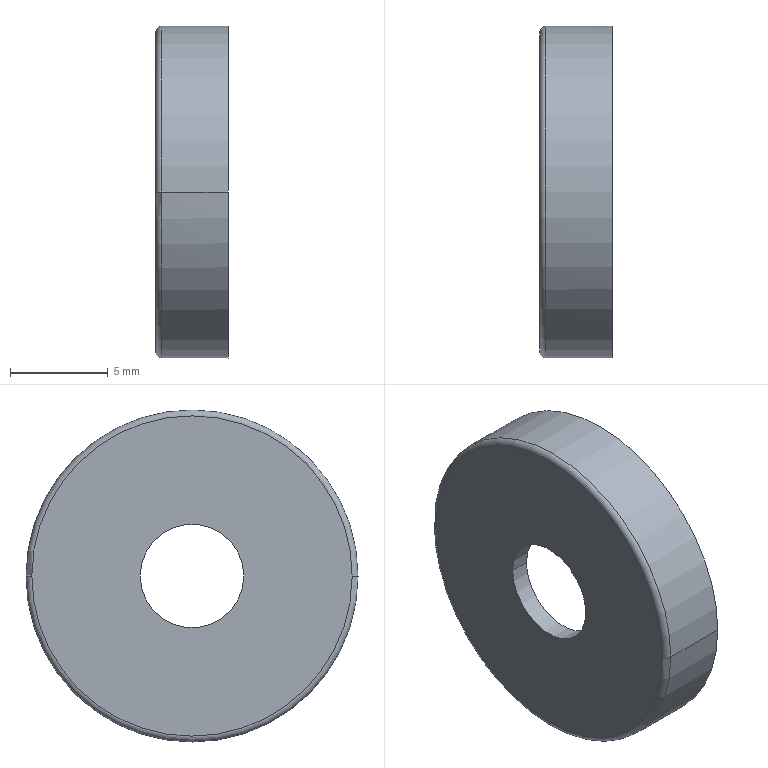Part | STEP file | ZHITUIZHOUCHEN_4_1_2_1_1 | 1 solid | 15 faces | box 3.7 x 17 x 17 mm | volume 365.454 mm3 | cylinder 6 | torus 4 | plane 3 | cone 2 | commonest cylinder face diameters 5.3 x2 14.5 x2 17 x2
STEP:
#1=CARTESIAN_POINT('',(0.,0.,0.));
#2=DIRECTION('',(0.,0.,1.));
#3=DIRECTION('',(1.,0.,0.));
#4=AXIS2_PLACEMENT_3D('',#1,#2,#3);
#5=CARTESIAN_POINT('',(0.,8.2,0.05125));
#6=VERTEX_POINT('',#5);
#7=CARTESIAN_POINT('',(0.,8.2,0.));
#8=VERTEX_POINT('',#7);
#9=CARTESIAN_POINT('',(0.,0.,0.));
#10=DIRECTION('',(-1.,0.,0.));
#11=DIRECTION('',(0.,1.,0.006251));
#12=AXIS2_PLACEMENT_3D('',#9,#10,#11);
#13=CIRCLE('',#12,8.2);
#14=EDGE_CURVE('',#6,#8,#13,.T.);
#15=ORIENTED_EDGE('',*,*,#14,.F.);
#16=CARTESIAN_POINT('',(0.,-8.2,0.));
#17=VERTEX_POINT('',#16);
#18=CARTESIAN_POINT('',(0.,0.,0.));
#19=DIRECTION('',(1.,0.,0.));
#20=DIRECTION('',(0.,1.,0.006251));
#21=AXIS2_PLACEMENT_3D('',#18,#19,#20);
#22=CIRCLE('',#21,8.2);
#23=EDGE_CURVE('',#6,#17,#22,.T.);
#24=ORIENTED_EDGE('',*,*,#23,.T.);
#25=CARTESIAN_POINT('',(0.,-8.2,-0.05125));
#26=VERTEX_POINT('',#25);
#27=CARTESIAN_POINT('',(0.,0.,0.));
#28=DIRECTION('',(-1.,0.,0.));
#29=DIRECTION('',(0.,-1.,-0.006251));
#30=AXIS2_PLACEMENT_3D('',#27,#28,#29);
#31=CIRCLE('',#30,8.2);
#32=EDGE_CURVE('',#26,#17,#31,.T.);
#33=ORIENTED_EDGE('',*,*,#32,.F.);
#34=CARTESIAN_POINT('',(0.,0.,0.));
#35=DIRECTION('',(1.,0.,0.));
#36=DIRECTION('',(0.,-1.,-0.006251));
#37=AXIS2_PLACEMENT_3D('',#34,#35,#36);
#38=CIRCLE('',#37,8.2);
#39=EDGE_CURVE('',#26,#8,#38,.T.);
#40=ORIENTED_EDGE('',*,*,#39,.T.);
#41=EDGE_LOOP('',(#15,#24,#33,#40));
#42=FACE_OUTER_BOUND('',#41,.F.);
#43=CARTESIAN_POINT('',(0.,2.65,0.));
#44=VERTEX_POINT('',#43);
#45=CARTESIAN_POINT('',(0.,-2.65,0.));
#46=VERTEX_POINT('',#45);
#47=CARTESIAN_POINT('',(0.,0.,0.));
#48=DIRECTION('',(-1.,0.,0.));
#49=DIRECTION('',(0.,1.,0.));
#50=AXIS2_PLACEMENT_3D('',#47,#48,#49);
#51=CIRCLE('',#50,2.65);
#52=EDGE_CURVE('',#44,#46,#51,.T.);
#53=ORIENTED_EDGE('',*,*,#52,.T.);
#54=CARTESIAN_POINT('',(0.,0.,0.));
#55=DIRECTION('',(-1.,0.,0.));
#56=DIRECTION('',(0.,-1.,0.));
#57=AXIS2_PLACEMENT_3D('',#54,#55,#56);
#58=CIRCLE('',#57,2.65);
#59=EDGE_CURVE('',#46,#44,#58,.T.);
#60=ORIENTED_EDGE('',*,*,#59,.T.);
#61=EDGE_LOOP('',(#53,#60));
#62=FACE_BOUND('',#61,.F.);
#63=CARTESIAN_POINT('',(0.,0.,0.));
#64=DIRECTION('',(1.,0.,0.));
#65=DIRECTION('',(0.,-1.,0.));
#66=AXIS2_PLACEMENT_3D('',#63,#64,#65);
#67=PLANE('',#66);
#68=ADVANCED_FACE('',(#42,#62),#67,.F.);
#69=ORIENTED_EDGE('',*,*,#23,.F.);
#70=ORIENTED_EDGE('',*,*,#14,.T.);
#71=CARTESIAN_POINT('',(0.3,8.5,0.));
#72=VERTEX_POINT('',#71);
#73=CARTESIAN_POINT('',(0.3,8.2,0.));
#74=DIRECTION('',(0.,0.,-1.));
#75=DIRECTION('',(-1.,0.,0.));
#76=AXIS2_PLACEMENT_3D('',#73,#74,#75);
#77=CIRCLE('',#76,0.3);
#78=EDGE_CURVE('',#8,#72,#77,.T.);
#79=ORIENTED_EDGE('',*,*,#78,.T.);
#80=CARTESIAN_POINT('',(0.3,8.5,0.05313));
#81=VERTEX_POINT('',#80);
#82=CARTESIAN_POINT('',(0.3,0.,0.));
#83=DIRECTION('',(1.,0.,0.));
#84=DIRECTION('',(0.,1.,0.));
#85=AXIS2_PLACEMENT_3D('',#82,#83,#84);
#86=CIRCLE('',#85,8.5);
#87=EDGE_CURVE('',#72,#81,#86,.T.);
#88=ORIENTED_EDGE('',*,*,#87,.T.);
#89=CARTESIAN_POINT('',(0.3,-8.5,0.));
#90=VERTEX_POINT('',#89);
#91=CARTESIAN_POINT('',(0.3,0.,0.));
#92=DIRECTION('',(1.,0.,0.));
#93=DIRECTION('',(0.,1.,0.006251));
#94=AXIS2_PLACEMENT_3D('',#91,#92,#93);
#95=CIRCLE('',#94,8.5);
#96=EDGE_CURVE('',#81,#90,#95,.T.);
#97=ORIENTED_EDGE('',*,*,#96,.T.);
#98=CARTESIAN_POINT('',(0.3,-8.2,0.));
#99=DIRECTION('',(0.,0.,1.));
#100=DIRECTION('',(-1.,0.,0.));
#101=AXIS2_PLACEMENT_3D('',#98,#99,#100);
#102=CIRCLE('',#101,0.3);
#103=EDGE_CURVE('',#17,#90,#102,.T.);
#104=ORIENTED_EDGE('',*,*,#103,.F.);
#105=EDGE_LOOP('',(#69,#70,#79,#88,#97,#104));
#106=FACE_OUTER_BOUND('',#105,.F.);
#107=CARTESIAN_POINT('',(0.3,0.,0.));
#108=DIRECTION('',(1.,0.,0.));
#109=DIRECTION('',(0.,-1.,-0.006251));
#110=AXIS2_PLACEMENT_3D('',#107,#108,#109);
#111=TOROIDAL_SURFACE('',#110,8.2,0.3);
#112=ADVANCED_FACE('',(#106),#111,.T.);
#113=ORIENTED_EDGE('',*,*,#39,.F.);
#114=ORIENTED_EDGE('',*,*,#32,.T.);
#115=ORIENTED_EDGE('',*,*,#103,.T.);
#116=CARTESIAN_POINT('',(0.3,-8.5,-0.05313));
#117=VERTEX_POINT('',#116);
#118=CARTESIAN_POINT('',(0.3,0.,0.));
#119=DIRECTION('',(1.,0.,0.));
#120=DIRECTION('',(0.,-1.,0.));
#121=AXIS2_PLACEMENT_3D('',#118,#119,#120);
#122=CIRCLE('',#121,8.5);
#123=EDGE_CURVE('',#90,#117,#122,.T.);
#124=ORIENTED_EDGE('',*,*,#123,.T.);
#125=CARTESIAN_POINT('',(0.3,0.,0.));
#126=DIRECTION('',(1.,0.,0.));
#127=DIRECTION('',(0.,-1.,-0.006251));
#128=AXIS2_PLACEMENT_3D('',#125,#126,#127);
#129=CIRCLE('',#128,8.5);
#130=EDGE_CURVE('',#117,#72,#129,.T.);
#131=ORIENTED_EDGE('',*,*,#130,.T.);
#132=ORIENTED_EDGE('',*,*,#78,.F.);
#133=EDGE_LOOP('',(#113,#114,#115,#124,#131,#132));
#134=FACE_OUTER_BOUND('',#133,.F.);
#135=CARTESIAN_POINT('',(0.3,0.,0.));
#136=DIRECTION('',(1.,0.,0.));
#137=DIRECTION('',(0.,1.,0.006251));
#138=AXIS2_PLACEMENT_3D('',#135,#136,#137);
#139=TOROIDAL_SURFACE('',#138,8.2,0.3);
#140=ADVANCED_FACE('',(#134),#139,.T.);
#141=ORIENTED_EDGE('',*,*,#130,.F.);
#142=ORIENTED_EDGE('',*,*,#123,.F.);
#143=CARTESIAN_POINT('',(3.7,-8.5,0.));
#144=VERTEX_POINT('',#143);
#145=CARTESIAN_POINT('',(0.3,-8.5,0.));
#146=DIRECTION('',(1.,0.,0.));
#147=VECTOR('',#146,3.4);
#148=LINE('',#145,#147);
#149=EDGE_CURVE('',#90,#144,#148,.T.);
#150=ORIENTED_EDGE('',*,*,#149,.T.);
#151=CARTESIAN_POINT('',(3.7,8.5,0.));
#152=VERTEX_POINT('',#151);
#153=CARTESIAN_POINT('',(3.7,0.,0.));
#154=DIRECTION('',(-1.,0.,0.));
#155=DIRECTION('',(0.,1.,0.));
#156=AXIS2_PLACEMENT_3D('',#153,#154,#155);
#157=CIRCLE('',#156,8.5);
#158=EDGE_CURVE('',#152,#144,#157,.T.);
#159=ORIENTED_EDGE('',*,*,#158,.F.);
#160=CARTESIAN_POINT('',(0.3,8.5,0.));
#161=DIRECTION('',(1.,0.,0.));
#162=VECTOR('',#161,3.4);
#163=LINE('',#160,#162);
#164=EDGE_CURVE('',#72,#152,#163,.T.);
#165=ORIENTED_EDGE('',*,*,#164,.F.);
#166=EDGE_LOOP('',(#141,#142,#150,#159,#165));
#167=FACE_OUTER_BOUND('',#166,.F.);
#168=CARTESIAN_POINT('',(0.,0.,0.));
#169=DIRECTION('',(1.,0.,0.));
#170=DIRECTION('',(0.,-1.,0.));
#171=AXIS2_PLACEMENT_3D('',#168,#169,#170);
#172=CYLINDRICAL_SURFACE('',#171,8.5);
#173=ADVANCED_FACE('',(#167),#172,.T.);
#174=ORIENTED_EDGE('',*,*,#96,.F.);
#175=ORIENTED_EDGE('',*,*,#87,.F.);
#176=ORIENTED_EDGE('',*,*,#164,.T.);
#177=CARTESIAN_POINT('',(3.7,0.,0.));
#178=DIRECTION('',(-1.,0.,0.));
#179=DIRECTION('',(0.,-1.,0.));
#180=AXIS2_PLACEMENT_3D('',#177,#178,#179);
#181=CIRCLE('',#180,8.5);
#182=EDGE_CURVE('',#144,#152,#181,.T.);
#183=ORIENTED_EDGE('',*,*,#182,.F.);
#184=ORIENTED_EDGE('',*,*,#149,.F.);
#185=EDGE_LOOP('',(#174,#175,#176,#183,#184));
#186=FACE_OUTER_BOUND('',#185,.F.);
#187=CARTESIAN_POINT('',(0.,0.,0.));
#188=DIRECTION('',(1.,0.,0.));
#189=DIRECTION('',(0.,-1.,0.));
#190=AXIS2_PLACEMENT_3D('',#187,#188,#189);
#191=CYLINDRICAL_SURFACE('',#190,8.5);
#192=ADVANCED_FACE('',(#186),#191,.T.);
#193=ORIENTED_EDGE('',*,*,#158,.T.);
#194=ORIENTED_EDGE('',*,*,#182,.T.);
#195=EDGE_LOOP('',(#193,#194));
#196=FACE_OUTER_BOUND('',#195,.F.);
#197=CARTESIAN_POINT('',(3.7,7.75,0.));
#198=VERTEX_POINT('',#197);
#199=CARTESIAN_POINT('',(3.7,0.,7.75));
#200=VERTEX_POINT('',#199);
#201=CARTESIAN_POINT('',(3.7,0.,0.));
#202=DIRECTION('',(1.,0.,0.));
#203=DIRECTION('',(0.,1.,0.));
#204=AXIS2_PLACEMENT_3D('',#201,#202,#203);
#205=CIRCLE('',#204,7.75);
#206=EDGE_CURVE('',#198,#200,#205,.T.);
#207=ORIENTED_EDGE('',*,*,#206,.T.);
#208=CARTESIAN_POINT('',(3.7,-7.75,0.));
#209=VERTEX_POINT('',#208);
#210=CARTESIAN_POINT('',(3.7,0.,0.));
#211=DIRECTION('',(1.,0.,0.));
#212=DIRECTION('',(0.,0.,1.));
#213=AXIS2_PLACEMENT_3D('',#210,#211,#212);
#214=CIRCLE('',#213,7.75);
#215=EDGE_CURVE('',#200,#209,#214,.T.);
#216=ORIENTED_EDGE('',*,*,#215,.T.);
#217=CARTESIAN_POINT('',(3.7,0.,-7.75));
#218=VERTEX_POINT('',#217);
#219=CARTESIAN_POINT('',(3.7,0.,0.));
#220=DIRECTION('',(1.,0.,0.));
#221=DIRECTION('',(0.,-1.,0.));
#222=AXIS2_PLACEMENT_3D('',#219,#220,#221);
#223=CIRCLE('',#222,7.75);
#224=EDGE_CURVE('',#209,#218,#223,.T.);
#225=ORIENTED_EDGE('',*,*,#224,.T.);
#226=CARTESIAN_POINT('',(3.7,0.,0.));
#227=DIRECTION('',(1.,0.,0.));
#228=DIRECTION('',(0.,0.,-1.));
#229=AXIS2_PLACEMENT_3D('',#226,#227,#228);
#230=CIRCLE('',#229,7.75);
#231=EDGE_CURVE('',#218,#198,#230,.T.);
#232=ORIENTED_EDGE('',*,*,#231,.T.);
#233=EDGE_LOOP('',(#207,#216,#225,#232));
#234=FACE_BOUND('',#233,.F.);
#235=CARTESIAN_POINT('',(3.7,0.,0.));
#236=DIRECTION('',(1.,0.,0.));
#237=DIRECTION('',(0.,-1.,0.));
#238=AXIS2_PLACEMENT_3D('',#235,#236,#237);
#239=PLANE('',#238);
#240=ADVANCED_FACE('',(#196,#234),#239,.T.);
#241=ORIENTED_EDGE('',*,*,#215,.F.);
#242=ORIENTED_EDGE('',*,*,#206,.F.);
#243=CARTESIAN_POINT('',(3.2,7.25,0.000000001));
#244=VERTEX_POINT('',#243);
#245=CARTESIAN_POINT('',(3.7,7.75,0.));
#246=DIRECTION('',(-0.7071,-0.7071,0.));
#247=VECTOR('',#246,0.7071);
#248=LINE('',#245,#247);
#249=EDGE_CURVE('',#198,#244,#248,.T.);
#250=ORIENTED_EDGE('',*,*,#249,.T.);
#251=CARTESIAN_POINT('',(3.2,-0.000000001,7.25));
#252=VERTEX_POINT('',#251);
#253=CARTESIAN_POINT('',(3.2,0.,0.));
#254=DIRECTION('',(1.,0.,0.));
#255=DIRECTION('',(0.,1.,0.));
#256=AXIS2_PLACEMENT_3D('',#253,#254,#255);
#257=CIRCLE('',#256,7.25);
#258=EDGE_CURVE('',#244,#252,#257,.T.);
#259=ORIENTED_EDGE('',*,*,#258,.T.);
#260=CARTESIAN_POINT('',(3.2,-7.25,0.));
#261=VERTEX_POINT('',#260);
#262=CARTESIAN_POINT('',(3.2,0.,0.));
#263=DIRECTION('',(1.,0.,0.));
#264=DIRECTION('',(0.,0.,1.));
#265=AXIS2_PLACEMENT_3D('',#262,#263,#264);
#266=CIRCLE('',#265,7.25);
#267=EDGE_CURVE('',#252,#261,#266,.T.);
#268=ORIENTED_EDGE('',*,*,#267,.T.);
#269=CARTESIAN_POINT('',(3.7,-7.75,0.));
#270=DIRECTION('',(-0.7071,0.7071,0.));
#271=VECTOR('',#270,0.7071);
#272=LINE('',#269,#271);
#273=EDGE_CURVE('',#209,#261,#272,.T.);
#274=ORIENTED_EDGE('',*,*,#273,.F.);
#275=EDGE_LOOP('',(#241,#242,#250,#259,#268,#274));
#276=FACE_OUTER_BOUND('',#275,.F.);
#277=CARTESIAN_POINT('',(3.45,0.,0.));
#278=DIRECTION('',(1.,0.,0.));
#279=DIRECTION('',(0.,0.,-1.));
#280=AXIS2_PLACEMENT_3D('',#277,#278,#279);
#281=CONICAL_SURFACE('',#280,7.5,45.);
#282=ADVANCED_FACE('',(#276),#281,.F.);
#283=ORIENTED_EDGE('',*,*,#231,.F.);
#284=ORIENTED_EDGE('',*,*,#224,.F.);
#285=ORIENTED_EDGE('',*,*,#273,.T.);
#286=CARTESIAN_POINT('',(3.2,0.,-7.25));
#287=VERTEX_POINT('',#286);
#288=CARTESIAN_POINT('',(3.2,0.,0.));
#289=DIRECTION('',(1.,0.,0.));
#290=DIRECTION('',(0.,-1.,0.));
#291=AXIS2_PLACEMENT_3D('',#288,#289,#290);
#292=CIRCLE('',#291,7.25);
#293=EDGE_CURVE('',#261,#287,#292,.T.);
#294=ORIENTED_EDGE('',*,*,#293,.T.);
#295=CARTESIAN_POINT('',(3.2,0.,0.));
#296=DIRECTION('',(1.,0.,0.));
#297=DIRECTION('',(0.,0.,-1.));
#298=AXIS2_PLACEMENT_3D('',#295,#296,#297);
#299=CIRCLE('',#298,7.25);
#300=EDGE_CURVE('',#287,#244,#299,.T.);
#301=ORIENTED_EDGE('',*,*,#300,.T.);
#302=ORIENTED_EDGE('',*,*,#249,.F.);
#303=EDGE_LOOP('',(#283,#284,#285,#294,#301,#302));
#304=FACE_OUTER_BOUND('',#303,.F.);
#305=CARTESIAN_POINT('',(3.45,0.,0.));
#306=DIRECTION('',(1.,0.,0.));
#307=DIRECTION('',(0.,0.,-1.));
#308=AXIS2_PLACEMENT_3D('',#305,#306,#307);
#309=CONICAL_SURFACE('',#308,7.5,45.);
#310=ADVANCED_FACE('',(#304),#309,.F.);
#311=CARTESIAN_POINT('',(1.2,-7.25,-0.05313));
#312=VERTEX_POINT('',#311);
#313=CARTESIAN_POINT('',(1.2,-7.25,0.));
#314=VERTEX_POINT('',#313);
#315=CARTESIAN_POINT('',(1.2,0.,0.));
#316=DIRECTION('',(-1.,0.,0.));
#317=DIRECTION('',(0.,-1.,-0.007328));
#318=AXIS2_PLACEMENT_3D('',#315,#316,#317);
#319=CIRCLE('',#318,7.25);
#320=EDGE_CURVE('',#312,#314,#319,.T.);
#321=ORIENTED_EDGE('',*,*,#320,.F.);
#322=CARTESIAN_POINT('',(1.2,7.25,0.));
#323=VERTEX_POINT('',#322);
#324=CARTESIAN_POINT('',(1.2,0.,0.));
#325=DIRECTION('',(-1.,0.,0.));
#326=DIRECTION('',(0.,1.,0.));
#327=AXIS2_PLACEMENT_3D('',#324,#325,#326);
#328=CIRCLE('',#327,7.25);
#329=EDGE_CURVE('',#323,#312,#328,.T.);
#330=ORIENTED_EDGE('',*,*,#329,.F.);
#331=CARTESIAN_POINT('',(3.2,7.25,0.000000001));
#332=DIRECTION('',(-1.,0.,0.));
#333=VECTOR('',#332,2.);
#334=LINE('',#331,#333);
#335=EDGE_CURVE('',#244,#323,#334,.T.);
#336=ORIENTED_EDGE('',*,*,#335,.F.);
#337=ORIENTED_EDGE('',*,*,#300,.F.);
#338=ORIENTED_EDGE('',*,*,#293,.F.);
#339=CARTESIAN_POINT('',(3.2,-7.25,0.));
#340=DIRECTION('',(-1.,0.,0.));
#341=VECTOR('',#340,2.);
#342=LINE('',#339,#341);
#343=EDGE_CURVE('',#261,#314,#342,.T.);
#344=ORIENTED_EDGE('',*,*,#343,.T.);
#345=EDGE_LOOP('',(#321,#330,#336,#337,#338,#344));
#346=FACE_OUTER_BOUND('',#345,.F.);
#347=CARTESIAN_POINT('',(3.7,0.,0.));
#348=DIRECTION('',(1.,0.,0.));
#349=DIRECTION('',(0.,-1.,0.));
#350=AXIS2_PLACEMENT_3D('',#347,#348,#349);
#351=CYLINDRICAL_SURFACE('',#350,7.25);
#352=ADVANCED_FACE('',(#346),#351,.F.);
#353=CARTESIAN_POINT('',(1.,-7.05,0.));
#354=VERTEX_POINT('',#353);
#355=CARTESIAN_POINT('',(1.,-7.05,-0.05166));
#356=VERTEX_POINT('',#355);
#357=CARTESIAN_POINT('',(1.,0.,0.));
#358=DIRECTION('',(1.,0.,0.));
#359=DIRECTION('',(0.,-1.,0.));
#360=AXIS2_PLACEMENT_3D('',#357,#358,#359);
#361=CIRCLE('',#360,7.05);
#362=EDGE_CURVE('',#354,#356,#361,.T.);
#363=ORIENTED_EDGE('',*,*,#362,.T.);
#364=CARTESIAN_POINT('',(1.,7.05,0.));
#365=VERTEX_POINT('',#364);
#366=CARTESIAN_POINT('',(1.,0.,0.));
#367=DIRECTION('',(-1.,0.,0.));
#368=DIRECTION('',(0.,1.,0.));
#369=AXIS2_PLACEMENT_3D('',#366,#367,#368);
#370=CIRCLE('',#369,7.05);
#371=EDGE_CURVE('',#365,#356,#370,.T.);
#372=ORIENTED_EDGE('',*,*,#371,.F.);
#373=CARTESIAN_POINT('',(1.2,7.05,0.));
#374=DIRECTION('',(0.,0.,-1.));
#375=DIRECTION('',(-1.,0.,0.));
#376=AXIS2_PLACEMENT_3D('',#373,#374,#375);
#377=CIRCLE('',#376,0.2);
#378=EDGE_CURVE('',#365,#323,#377,.T.);
#379=ORIENTED_EDGE('',*,*,#378,.T.);
#380=ORIENTED_EDGE('',*,*,#329,.T.);
#381=ORIENTED_EDGE('',*,*,#320,.T.);
#382=CARTESIAN_POINT('',(1.2,-7.05,0.));
#383=DIRECTION('',(0.,0.,1.));
#384=DIRECTION('',(-1.,0.,0.));
#385=AXIS2_PLACEMENT_3D('',#382,#383,#384);
#386=CIRCLE('',#385,0.2);
#387=EDGE_CURVE('',#354,#314,#386,.T.);
#388=ORIENTED_EDGE('',*,*,#387,.F.);
#389=EDGE_LOOP('',(#363,#372,#379,#380,#381,#388));
#390=FACE_OUTER_BOUND('',#389,.F.);
#391=CARTESIAN_POINT('',(1.2,0.,0.));
#392=DIRECTION('',(1.,0.,0.));
#393=DIRECTION('',(0.,1.,0.007328));
#394=AXIS2_PLACEMENT_3D('',#391,#392,#393);
#395=TOROIDAL_SURFACE('',#394,7.05,0.2);
#396=ADVANCED_FACE('',(#390),#395,.F.);
#397=CARTESIAN_POINT('',(1.,7.05,0.05166));
#398=VERTEX_POINT('',#397);
#399=CARTESIAN_POINT('',(1.,0.,0.));
#400=DIRECTION('',(-1.,0.,0.));
#401=DIRECTION('',(0.,-1.,0.));
#402=AXIS2_PLACEMENT_3D('',#399,#400,#401);
#403=CIRCLE('',#402,7.05);
#404=EDGE_CURVE('',#354,#398,#403,.T.);
#405=ORIENTED_EDGE('',*,*,#404,.T.);
#406=CARTESIAN_POINT('',(1.,0.,0.));
#407=DIRECTION('',(1.,0.,0.));
#408=DIRECTION('',(0.,1.,0.));
#409=AXIS2_PLACEMENT_3D('',#406,#407,#408);
#410=CIRCLE('',#409,7.05);
#411=EDGE_CURVE('',#365,#398,#410,.T.);
#412=ORIENTED_EDGE('',*,*,#411,.F.);
#413=ORIENTED_EDGE('',*,*,#371,.T.);
#414=ORIENTED_EDGE('',*,*,#362,.F.);
#415=EDGE_LOOP('',(#405,#412,#413,#414));
#416=FACE_OUTER_BOUND('',#415,.F.);
#417=CARTESIAN_POINT('',(1.,-2.65,0.));
#418=VERTEX_POINT('',#417);
#419=CARTESIAN_POINT('',(1.,2.65,0.));
#420=VERTEX_POINT('',#419);
#421=CARTESIAN_POINT('',(1.,0.,0.));
#422=DIRECTION('',(1.,0.,0.));
#423=DIRECTION('',(0.,-1.,0.));
#424=AXIS2_PLACEMENT_3D('',#421,#422,#423);
#425=CIRCLE('',#424,2.65);
#426=EDGE_CURVE('',#418,#420,#425,.T.);
#427=ORIENTED_EDGE('',*,*,#426,.T.);
#428=CARTESIAN_POINT('',(1.,0.,0.));
#429=DIRECTION('',(1.,0.,0.));
#430=DIRECTION('',(0.,1.,0.));
#431=AXIS2_PLACEMENT_3D('',#428,#429,#430);
#432=CIRCLE('',#431,2.65);
#433=EDGE_CURVE('',#420,#418,#432,.T.);
#434=ORIENTED_EDGE('',*,*,#433,.T.);
#435=EDGE_LOOP('',(#427,#434));
#436=FACE_BOUND('',#435,.F.);
#437=CARTESIAN_POINT('',(1.,0.,0.));
#438=DIRECTION('',(1.,0.,0.));
#439=DIRECTION('',(0.,-1.,0.));
#440=AXIS2_PLACEMENT_3D('',#437,#438,#439);
#441=PLANE('',#440);
#442=ADVANCED_FACE('',(#416,#436),#441,.T.);
#443=ORIENTED_EDGE('',*,*,#411,.T.);
#444=ORIENTED_EDGE('',*,*,#404,.F.);
#445=ORIENTED_EDGE('',*,*,#387,.T.);
#446=CARTESIAN_POINT('',(1.2,7.25,0.05313));
#447=VERTEX_POINT('',#446);
#448=CARTESIAN_POINT('',(1.2,0.,0.));
#449=DIRECTION('',(-1.,0.,0.));
#450=DIRECTION('',(0.,-1.,0.));
#451=AXIS2_PLACEMENT_3D('',#448,#449,#450);
#452=CIRCLE('',#451,7.25);
#453=EDGE_CURVE('',#314,#447,#452,.T.);
#454=ORIENTED_EDGE('',*,*,#453,.T.);
#455=CARTESIAN_POINT('',(1.2,0.,0.));
#456=DIRECTION('',(-1.,0.,0.));
#457=DIRECTION('',(0.,1.,0.007328));
#458=AXIS2_PLACEMENT_3D('',#455,#456,#457);
#459=CIRCLE('',#458,7.25);
#460=EDGE_CURVE('',#447,#323,#459,.T.);
#461=ORIENTED_EDGE('',*,*,#460,.T.);
#462=ORIENTED_EDGE('',*,*,#378,.F.);
#463=EDGE_LOOP('',(#443,#444,#445,#454,#461,#462));
#464=FACE_OUTER_BOUND('',#463,.F.);
#465=CARTESIAN_POINT('',(1.2,0.,0.));
#466=DIRECTION('',(1.,0.,0.));
#467=DIRECTION('',(0.,-1.,-0.007328));
#468=AXIS2_PLACEMENT_3D('',#465,#466,#467);
#469=TOROIDAL_SURFACE('',#468,7.05,0.2);
#470=ADVANCED_FACE('',(#464),#469,.F.);
#471=ORIENTED_EDGE('',*,*,#460,.F.);
#472=ORIENTED_EDGE('',*,*,#453,.F.);
#473=ORIENTED_EDGE('',*,*,#343,.F.);
#474=ORIENTED_EDGE('',*,*,#267,.F.);
#475=ORIENTED_EDGE('',*,*,#258,.F.);
#476=ORIENTED_EDGE('',*,*,#335,.T.);
#477=EDGE_LOOP('',(#471,#472,#473,#474,#475,#476));
#478=FACE_OUTER_BOUND('',#477,.F.);
#479=CARTESIAN_POINT('',(3.7,0.,0.));
#480=DIRECTION('',(1.,0.,0.));
#481=DIRECTION('',(0.,-1.,0.));
#482=AXIS2_PLACEMENT_3D('',#479,#480,#481);
#483=CYLINDRICAL_SURFACE('',#482,7.25);
#484=ADVANCED_FACE('',(#478),#483,.F.);
#485=ORIENTED_EDGE('',*,*,#52,.F.);
#486=CARTESIAN_POINT('',(1.,2.65,0.));
#487=DIRECTION('',(-1.,0.,0.));
#488=VECTOR('',#487,1.);
#489=LINE('',#486,#488);
#490=EDGE_CURVE('',#420,#44,#489,.T.);
#491=ORIENTED_EDGE('',*,*,#490,.F.);
#492=ORIENTED_EDGE('',*,*,#426,.F.);
#493=CARTESIAN_POINT('',(1.,-2.65,0.));
#494=DIRECTION('',(-1.,0.,0.));
#495=VECTOR('',#494,1.);
#496=LINE('',#493,#495);
#497=EDGE_CURVE('',#418,#46,#496,.T.);
#498=ORIENTED_EDGE('',*,*,#497,.T.);
#499=EDGE_LOOP('',(#485,#491,#492,#498));
#500=FACE_OUTER_BOUND('',#499,.F.);
#501=CARTESIAN_POINT('',(1.,0.,0.));
#502=DIRECTION('',(1.,0.,0.));
#503=DIRECTION('',(0.,-1.,0.));
#504=AXIS2_PLACEMENT_3D('',#501,#502,#503);
#505=CYLINDRICAL_SURFACE('',#504,2.65);
#506=ADVANCED_FACE('',(#500),#505,.F.);
#507=ORIENTED_EDGE('',*,*,#59,.F.);
#508=ORIENTED_EDGE('',*,*,#497,.F.);
#509=ORIENTED_EDGE('',*,*,#433,.F.);
#510=ORIENTED_EDGE('',*,*,#490,.T.);
#511=EDGE_LOOP('',(#507,#508,#509,#510));
#512=FACE_OUTER_BOUND('',#511,.F.);
#513=CARTESIAN_POINT('',(1.,0.,0.));
#514=DIRECTION('',(1.,0.,0.));
#515=DIRECTION('',(0.,-1.,0.));
#516=AXIS2_PLACEMENT_3D('',#513,#514,#515);
#517=CYLINDRICAL_SURFACE('',#516,2.65);
#518=ADVANCED_FACE('',(#512),#517,.F.);
#519=CLOSED_SHELL('',(#68,#112,#140,#173,#192,#240,#282,#310,#352,#396,#442,#470,#484,#506,#518));
#520=MANIFOLD_SOLID_BREP('',#519);
#521=(LENGTH_UNIT()NAMED_UNIT(*)SI_UNIT(.MILLI.,.METRE.));
#522=UNCERTAINTY_MEASURE_WITH_UNIT(LENGTH_MEASURE(0.002433),#521,'','');
#523=(NAMED_UNIT(*)PLANE_ANGLE_UNIT()SI_UNIT($,.RADIAN.));
#524=PLANE_ANGLE_MEASURE_WITH_UNIT(PLANE_ANGLE_MEASURE(0.01745),#523);
#525=(CONVERSION_BASED_UNIT('DEGREE',#524)NAMED_UNIT(*)PLANE_ANGLE_UNIT());
#526=(NAMED_UNIT(*)SI_UNIT($,.STERADIAN.)SOLID_ANGLE_UNIT());
#527=(GEOMETRIC_REPRESENTATION_CONTEXT(3)GLOBAL_UNCERTAINTY_ASSIGNED_CONTEXT((#522))GLOBAL_UNIT_ASSIGNED_CONTEXT((#521,#525,#526))REPRESENTATION_CONTEXT('',''));
#528=ADVANCED_BREP_SHAPE_REPRESENTATION('',(#4,#520),#527);